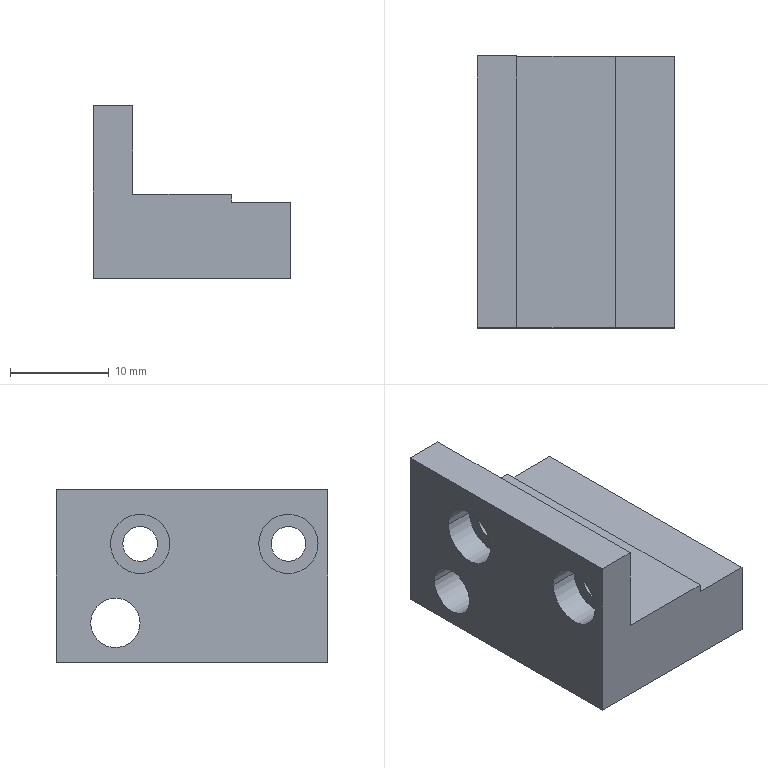Part | NX | 1 solid | 22 faces | box 20 x 27.5 x 17.5 mm | volume 4951 mm3 | plane 12 | cylinder 10 | commonest cylinder face diameters 3.5 x4 6 x4 5 x2
STEP:
#1=CARTESIAN_POINT('',(20.,5.5,-9.8));
#2=VERTEX_POINT('',#1);
#3=CARTESIAN_POINT('',(14.,5.5,-9.8));
#4=VERTEX_POINT('',#3);
#5=CARTESIAN_POINT('',(0.,5.5,-9.8));
#6=DIRECTION('',(-1.,0.,0.));
#7=VECTOR('',#6,1000.);
#8=LINE('',#5,#7);
#9=EDGE_CURVE('',#2,#4,#8,.T.);
#10=ORIENTED_EDGE('',*,*,#9,.T.);
#11=CARTESIAN_POINT('',(14.,5.5,-9.));
#12=VERTEX_POINT('',#11);
#13=CARTESIAN_POINT('',(14.,5.5,0.));
#14=DIRECTION('',(0.,0.,1.));
#15=VECTOR('',#14,1000.);
#16=LINE('',#13,#15);
#17=EDGE_CURVE('',#4,#12,#16,.T.);
#18=ORIENTED_EDGE('',*,*,#17,.T.);
#19=CARTESIAN_POINT('',(4.,5.5,-9.));
#20=VERTEX_POINT('',#19);
#21=CARTESIAN_POINT('',(0.,5.5,-9.));
#22=DIRECTION('',(1.,0.,0.));
#23=VECTOR('',#22,1000.);
#24=LINE('',#21,#23);
#25=EDGE_CURVE('',#20,#12,#24,.T.);
#26=ORIENTED_EDGE('',*,*,#25,.F.);
#27=CARTESIAN_POINT('',(4.,5.5,0.));
#28=VERTEX_POINT('',#27);
#29=CARTESIAN_POINT('',(4.,5.5,0.));
#30=DIRECTION('',(0.,0.,-1.));
#31=VECTOR('',#30,1000.);
#32=LINE('',#29,#31);
#33=EDGE_CURVE('',#28,#20,#32,.T.);
#34=ORIENTED_EDGE('',*,*,#33,.F.);
#35=CARTESIAN_POINT('',(0.,5.5,0.));
#36=VERTEX_POINT('',#35);
#37=CARTESIAN_POINT('',(0.,5.5,0.));
#38=DIRECTION('',(1.,0.,0.));
#39=VECTOR('',#38,1000.);
#40=LINE('',#37,#39);
#41=EDGE_CURVE('',#36,#28,#40,.T.);
#42=ORIENTED_EDGE('',*,*,#41,.F.);
#43=CARTESIAN_POINT('',(0.,5.5,-17.5));
#44=VERTEX_POINT('',#43);
#45=CARTESIAN_POINT('',(0.,5.5,0.));
#46=DIRECTION('',(0.,0.,1.));
#47=VECTOR('',#46,1000.);
#48=LINE('',#45,#47);
#49=EDGE_CURVE('',#44,#36,#48,.T.);
#50=ORIENTED_EDGE('',*,*,#49,.F.);
#51=CARTESIAN_POINT('',(20.,5.5,-17.5));
#52=VERTEX_POINT('',#51);
#53=CARTESIAN_POINT('',(0.,5.5,-17.5));
#54=DIRECTION('',(-1.,0.,0.));
#55=VECTOR('',#54,1000.);
#56=LINE('',#53,#55);
#57=EDGE_CURVE('',#52,#44,#56,.T.);
#58=ORIENTED_EDGE('',*,*,#57,.F.);
#59=CARTESIAN_POINT('',(20.,5.5,0.));
#60=DIRECTION('',(0.,0.,-1.));
#61=VECTOR('',#60,1000.);
#62=LINE('',#59,#61);
#63=EDGE_CURVE('',#2,#52,#62,.T.);
#64=ORIENTED_EDGE('',*,*,#63,.F.);
#65=EDGE_LOOP('',(#10,#18,#26,#34,#42,#50,#58,#64));
#66=FACE_BOUND('',#65,.T.);
#67=CARTESIAN_POINT('',(0.,5.5,0.));
#68=DIRECTION('',(0.,1.,0.));
#69=DIRECTION('',(1.,0.,0.));
#70=AXIS2_PLACEMENT_3D('',#67,#68,#69);
#71=PLANE('',#70);
#72=ADVANCED_FACE('',(#66),#71,.F.);
#73=ORIENTED_EDGE('',*,*,#9,.F.);
#74=CARTESIAN_POINT('',(20.,33.,-9.8));
#75=VERTEX_POINT('',#74);
#76=CARTESIAN_POINT('',(20.,0.,-9.8));
#77=DIRECTION('',(0.,-1.,0.));
#78=VECTOR('',#77,1000.);
#79=LINE('',#76,#78);
#80=EDGE_CURVE('',#75,#2,#79,.T.);
#81=ORIENTED_EDGE('',*,*,#80,.F.);
#82=CARTESIAN_POINT('',(14.,33.,-9.8));
#83=VERTEX_POINT('',#82);
#84=CARTESIAN_POINT('',(0.,33.,-9.8));
#85=DIRECTION('',(-1.,0.,0.));
#86=VECTOR('',#85,1000.);
#87=LINE('',#84,#86);
#88=EDGE_CURVE('',#75,#83,#87,.T.);
#89=ORIENTED_EDGE('',*,*,#88,.T.);
#90=CARTESIAN_POINT('',(14.,0.,-9.8));
#91=DIRECTION('',(0.,1.,0.));
#92=VECTOR('',#91,1000.);
#93=LINE('',#90,#92);
#94=EDGE_CURVE('',#4,#83,#93,.T.);
#95=ORIENTED_EDGE('',*,*,#94,.F.);
#96=EDGE_LOOP('',(#73,#81,#89,#95));
#97=FACE_BOUND('',#96,.T.);
#98=CARTESIAN_POINT('',(20.,34.,-9.8));
#99=DIRECTION('',(0.,0.,-1.));
#100=DIRECTION('',(0.,-1.,0.));
#101=AXIS2_PLACEMENT_3D('',#98,#99,#100);
#102=PLANE('',#101);
#103=ADVANCED_FACE('',(#97),#102,.F.);
#104=ORIENTED_EDGE('',*,*,#17,.F.);
#105=ORIENTED_EDGE('',*,*,#94,.T.);
#106=CARTESIAN_POINT('',(14.,33.,-9.));
#107=VERTEX_POINT('',#106);
#108=CARTESIAN_POINT('',(14.,33.,0.));
#109=DIRECTION('',(0.,0.,1.));
#110=VECTOR('',#109,1000.);
#111=LINE('',#108,#110);
#112=EDGE_CURVE('',#83,#107,#111,.T.);
#113=ORIENTED_EDGE('',*,*,#112,.T.);
#114=CARTESIAN_POINT('',(14.,0.,-9.));
#115=DIRECTION('',(0.,-1.,0.));
#116=VECTOR('',#115,1000.);
#117=LINE('',#114,#116);
#118=EDGE_CURVE('',#107,#12,#117,.T.);
#119=ORIENTED_EDGE('',*,*,#118,.T.);
#120=EDGE_LOOP('',(#104,#105,#113,#119));
#121=FACE_BOUND('',#120,.T.);
#122=CARTESIAN_POINT('',(14.,34.,-9.8));
#123=DIRECTION('',(-1.,0.,0.));
#124=DIRECTION('',(0.,0.,1.));
#125=AXIS2_PLACEMENT_3D('',#122,#123,#124);
#126=PLANE('',#125);
#127=ADVANCED_FACE('',(#121),#126,.F.);
#128=ORIENTED_EDGE('',*,*,#118,.F.);
#129=CARTESIAN_POINT('',(4.,33.,-9.));
#130=VERTEX_POINT('',#129);
#131=CARTESIAN_POINT('',(0.,33.,-9.));
#132=DIRECTION('',(1.,0.,0.));
#133=VECTOR('',#132,1000.);
#134=LINE('',#131,#133);
#135=EDGE_CURVE('',#130,#107,#134,.T.);
#136=ORIENTED_EDGE('',*,*,#135,.F.);
#137=CARTESIAN_POINT('',(4.,0.,-9.));
#138=DIRECTION('',(0.,1.,0.));
#139=VECTOR('',#138,1000.);
#140=LINE('',#137,#139);
#141=EDGE_CURVE('',#20,#130,#140,.T.);
#142=ORIENTED_EDGE('',*,*,#141,.F.);
#143=ORIENTED_EDGE('',*,*,#25,.T.);
#144=EDGE_LOOP('',(#128,#136,#142,#143));
#145=FACE_BOUND('',#144,.T.);
#146=CARTESIAN_POINT('',(4.,0.,-9.));
#147=DIRECTION('',(0.,0.,1.));
#148=DIRECTION('',(1.,0.,0.));
#149=AXIS2_PLACEMENT_3D('',#146,#147,#148);
#150=PLANE('',#149);
#151=ADVANCED_FACE('',(#145),#150,.T.);
#152=ORIENTED_EDGE('',*,*,#80,.T.);
#153=ORIENTED_EDGE('',*,*,#63,.T.);
#154=CARTESIAN_POINT('',(20.,33.,-17.5));
#155=VERTEX_POINT('',#154);
#156=CARTESIAN_POINT('',(20.,0.,-17.5));
#157=DIRECTION('',(0.,-1.,0.));
#158=VECTOR('',#157,1000.);
#159=LINE('',#156,#158);
#160=EDGE_CURVE('',#155,#52,#159,.T.);
#161=ORIENTED_EDGE('',*,*,#160,.F.);
#162=CARTESIAN_POINT('',(20.,33.,0.));
#163=DIRECTION('',(0.,0.,-1.));
#164=VECTOR('',#163,1000.);
#165=LINE('',#162,#164);
#166=EDGE_CURVE('',#75,#155,#165,.T.);
#167=ORIENTED_EDGE('',*,*,#166,.F.);
#168=EDGE_LOOP('',(#152,#153,#161,#167));
#169=FACE_BOUND('',#168,.T.);
#170=CARTESIAN_POINT('',(20.,29.5,-13.5));
#171=VERTEX_POINT('',#170);
#172=CARTESIAN_POINT('',(20.,24.5,-13.5));
#173=VERTEX_POINT('',#172);
#174=CARTESIAN_POINT('',(20.,27.,-13.5));
#175=DIRECTION('',(1.,0.,0.));
#176=DIRECTION('',(0.,1.,0.));
#177=AXIS2_PLACEMENT_3D('',#174,#175,#176);
#178=CIRCLE('',#177,2.5);
#179=EDGE_CURVE('',#171,#173,#178,.T.);
#180=ORIENTED_EDGE('',*,*,#179,.F.);
#181=CARTESIAN_POINT('',(20.,27.,-13.5));
#182=DIRECTION('',(1.,0.,0.));
#183=DIRECTION('',(0.,1.,0.));
#184=AXIS2_PLACEMENT_3D('',#181,#182,#183);
#185=CIRCLE('',#184,2.5);
#186=EDGE_CURVE('',#173,#171,#185,.T.);
#187=ORIENTED_EDGE('',*,*,#186,.F.);
#188=EDGE_LOOP('',(#180,#187));
#189=FACE_BOUND('',#188,.T.);
#190=CARTESIAN_POINT('',(20.,0.,-9.));
#191=DIRECTION('',(1.,0.,0.));
#192=DIRECTION('',(0.,1.,0.));
#193=AXIS2_PLACEMENT_3D('',#190,#191,#192);
#194=PLANE('',#193);
#195=ADVANCED_FACE('',(#169,#189),#194,.T.);
#196=ORIENTED_EDGE('',*,*,#41,.T.);
#197=CARTESIAN_POINT('',(4.,33.,0.));
#198=VERTEX_POINT('',#197);
#199=CARTESIAN_POINT('',(4.,0.,0.));
#200=DIRECTION('',(0.,-1.,0.));
#201=VECTOR('',#200,1000.);
#202=LINE('',#199,#201);
#203=EDGE_CURVE('',#198,#28,#202,.T.);
#204=ORIENTED_EDGE('',*,*,#203,.F.);
#205=CARTESIAN_POINT('',(0.,33.,0.));
#206=VERTEX_POINT('',#205);
#207=CARTESIAN_POINT('',(0.,33.,0.));
#208=DIRECTION('',(1.,0.,0.));
#209=VECTOR('',#208,1000.);
#210=LINE('',#207,#209);
#211=EDGE_CURVE('',#206,#198,#210,.T.);
#212=ORIENTED_EDGE('',*,*,#211,.F.);
#213=CARTESIAN_POINT('',(0.,0.,0.));
#214=DIRECTION('',(0.,1.,0.));
#215=VECTOR('',#214,1000.);
#216=LINE('',#213,#215);
#217=EDGE_CURVE('',#36,#206,#216,.T.);
#218=ORIENTED_EDGE('',*,*,#217,.F.);
#219=EDGE_LOOP('',(#196,#204,#212,#218));
#220=FACE_BOUND('',#219,.T.);
#221=CARTESIAN_POINT('',(0.,0.,0.));
#222=DIRECTION('',(0.,0.,1.));
#223=DIRECTION('',(1.,0.,0.));
#224=AXIS2_PLACEMENT_3D('',#221,#222,#223);
#225=PLANE('',#224);
#226=ADVANCED_FACE('',(#220),#225,.T.);
#227=ORIENTED_EDGE('',*,*,#33,.T.);
#228=ORIENTED_EDGE('',*,*,#141,.T.);
#229=CARTESIAN_POINT('',(4.,33.,0.));
#230=DIRECTION('',(0.,0.,-1.));
#231=VECTOR('',#230,1000.);
#232=LINE('',#229,#231);
#233=EDGE_CURVE('',#198,#130,#232,.T.);
#234=ORIENTED_EDGE('',*,*,#233,.F.);
#235=ORIENTED_EDGE('',*,*,#203,.T.);
#236=EDGE_LOOP('',(#227,#228,#234,#235));
#237=FACE_BOUND('',#236,.T.);
#238=CARTESIAN_POINT('',(4.,7.75,-5.5));
#239=VERTEX_POINT('',#238);
#240=CARTESIAN_POINT('',(4.,11.25,-5.5));
#241=VERTEX_POINT('',#240);
#242=CARTESIAN_POINT('',(4.,9.5,-5.5));
#243=DIRECTION('',(-1.,0.,0.));
#244=DIRECTION('',(0.,1.,0.));
#245=AXIS2_PLACEMENT_3D('',#242,#243,#244);
#246=CIRCLE('',#245,1.75);
#247=EDGE_CURVE('',#239,#241,#246,.T.);
#248=ORIENTED_EDGE('',*,*,#247,.T.);
#249=CARTESIAN_POINT('',(4.,9.5,-5.5));
#250=DIRECTION('',(-1.,0.,0.));
#251=DIRECTION('',(0.,1.,0.));
#252=AXIS2_PLACEMENT_3D('',#249,#250,#251);
#253=CIRCLE('',#252,1.75);
#254=EDGE_CURVE('',#241,#239,#253,.T.);
#255=ORIENTED_EDGE('',*,*,#254,.T.);
#256=EDGE_LOOP('',(#248,#255));
#257=FACE_BOUND('',#256,.T.);
#258=CARTESIAN_POINT('',(4.,26.25,-5.5));
#259=VERTEX_POINT('',#258);
#260=CARTESIAN_POINT('',(4.,22.75,-5.5));
#261=VERTEX_POINT('',#260);
#262=CARTESIAN_POINT('',(4.,24.5,-5.5));
#263=DIRECTION('',(-1.,0.,0.));
#264=DIRECTION('',(0.,1.,0.));
#265=AXIS2_PLACEMENT_3D('',#262,#263,#264);
#266=CIRCLE('',#265,1.75);
#267=EDGE_CURVE('',#259,#261,#266,.T.);
#268=ORIENTED_EDGE('',*,*,#267,.T.);
#269=CARTESIAN_POINT('',(4.,24.5,-5.5));
#270=DIRECTION('',(-1.,0.,0.));
#271=DIRECTION('',(0.,1.,0.));
#272=AXIS2_PLACEMENT_3D('',#269,#270,#271);
#273=CIRCLE('',#272,1.75);
#274=EDGE_CURVE('',#261,#259,#273,.T.);
#275=ORIENTED_EDGE('',*,*,#274,.T.);
#276=EDGE_LOOP('',(#268,#275));
#277=FACE_BOUND('',#276,.T.);
#278=CARTESIAN_POINT('',(4.,0.,0.));
#279=DIRECTION('',(1.,0.,0.));
#280=DIRECTION('',(0.,1.,0.));
#281=AXIS2_PLACEMENT_3D('',#278,#279,#280);
#282=PLANE('',#281);
#283=ADVANCED_FACE('',(#237,#257,#277),#282,.T.);
#284=ORIENTED_EDGE('',*,*,#57,.T.);
#285=CARTESIAN_POINT('',(0.,33.,-17.5));
#286=VERTEX_POINT('',#285);
#287=CARTESIAN_POINT('',(0.,0.,-17.5));
#288=DIRECTION('',(0.,-1.,0.));
#289=VECTOR('',#288,1000.);
#290=LINE('',#287,#289);
#291=EDGE_CURVE('',#286,#44,#290,.T.);
#292=ORIENTED_EDGE('',*,*,#291,.F.);
#293=CARTESIAN_POINT('',(0.,33.,-17.5));
#294=DIRECTION('',(-1.,0.,0.));
#295=VECTOR('',#294,1000.);
#296=LINE('',#293,#295);
#297=EDGE_CURVE('',#155,#286,#296,.T.);
#298=ORIENTED_EDGE('',*,*,#297,.F.);
#299=ORIENTED_EDGE('',*,*,#160,.T.);
#300=EDGE_LOOP('',(#284,#292,#298,#299));
#301=FACE_BOUND('',#300,.T.);
#302=CARTESIAN_POINT('',(20.,0.,-17.5));
#303=DIRECTION('',(0.,0.,-1.));
#304=DIRECTION('',(0.,-1.,0.));
#305=AXIS2_PLACEMENT_3D('',#302,#303,#304);
#306=PLANE('',#305);
#307=ADVANCED_FACE('',(#301),#306,.T.);
#308=ORIENTED_EDGE('',*,*,#49,.T.);
#309=ORIENTED_EDGE('',*,*,#217,.T.);
#310=CARTESIAN_POINT('',(0.,33.,0.));
#311=DIRECTION('',(0.,0.,1.));
#312=VECTOR('',#311,1000.);
#313=LINE('',#310,#312);
#314=EDGE_CURVE('',#286,#206,#313,.T.);
#315=ORIENTED_EDGE('',*,*,#314,.F.);
#316=ORIENTED_EDGE('',*,*,#291,.T.);
#317=EDGE_LOOP('',(#308,#309,#315,#316));
#318=FACE_BOUND('',#317,.T.);
#319=CARTESIAN_POINT('',(0.,12.5,-5.5));
#320=VERTEX_POINT('',#319);
#321=CARTESIAN_POINT('',(0.,6.5,-5.5));
#322=VERTEX_POINT('',#321);
#323=CARTESIAN_POINT('',(0.,9.5,-5.5));
#324=DIRECTION('',(-1.,0.,0.));
#325=DIRECTION('',(0.,1.,0.));
#326=AXIS2_PLACEMENT_3D('',#323,#324,#325);
#327=CIRCLE('',#326,3.);
#328=EDGE_CURVE('',#320,#322,#327,.T.);
#329=ORIENTED_EDGE('',*,*,#328,.F.);
#330=CARTESIAN_POINT('',(0.,9.5,-5.5));
#331=DIRECTION('',(-1.,0.,0.));
#332=DIRECTION('',(0.,1.,0.));
#333=AXIS2_PLACEMENT_3D('',#330,#331,#332);
#334=CIRCLE('',#333,3.);
#335=EDGE_CURVE('',#322,#320,#334,.T.);
#336=ORIENTED_EDGE('',*,*,#335,.F.);
#337=EDGE_LOOP('',(#329,#336));
#338=FACE_BOUND('',#337,.T.);
#339=CARTESIAN_POINT('',(0.,24.5,-13.5));
#340=VERTEX_POINT('',#339);
#341=CARTESIAN_POINT('',(0.,29.5,-13.5));
#342=VERTEX_POINT('',#341);
#343=CARTESIAN_POINT('',(0.,27.,-13.5));
#344=DIRECTION('',(1.,0.,0.));
#345=DIRECTION('',(0.,1.,0.));
#346=AXIS2_PLACEMENT_3D('',#343,#344,#345);
#347=CIRCLE('',#346,2.5);
#348=EDGE_CURVE('',#340,#342,#347,.T.);
#349=ORIENTED_EDGE('',*,*,#348,.T.);
#350=CARTESIAN_POINT('',(0.,27.,-13.5));
#351=DIRECTION('',(1.,0.,0.));
#352=DIRECTION('',(0.,1.,0.));
#353=AXIS2_PLACEMENT_3D('',#350,#351,#352);
#354=CIRCLE('',#353,2.5);
#355=EDGE_CURVE('',#342,#340,#354,.T.);
#356=ORIENTED_EDGE('',*,*,#355,.T.);
#357=EDGE_LOOP('',(#349,#356));
#358=FACE_BOUND('',#357,.T.);
#359=CARTESIAN_POINT('',(0.,21.5,-5.5));
#360=VERTEX_POINT('',#359);
#361=CARTESIAN_POINT('',(0.,27.5,-5.5));
#362=VERTEX_POINT('',#361);
#363=CARTESIAN_POINT('',(0.,24.5,-5.5));
#364=DIRECTION('',(-1.,0.,0.));
#365=DIRECTION('',(0.,1.,0.));
#366=AXIS2_PLACEMENT_3D('',#363,#364,#365);
#367=CIRCLE('',#366,3.);
#368=EDGE_CURVE('',#360,#362,#367,.T.);
#369=ORIENTED_EDGE('',*,*,#368,.F.);
#370=CARTESIAN_POINT('',(0.,24.5,-5.5));
#371=DIRECTION('',(-1.,0.,0.));
#372=DIRECTION('',(0.,1.,0.));
#373=AXIS2_PLACEMENT_3D('',#370,#371,#372);
#374=CIRCLE('',#373,3.);
#375=EDGE_CURVE('',#362,#360,#374,.T.);
#376=ORIENTED_EDGE('',*,*,#375,.F.);
#377=EDGE_LOOP('',(#369,#376));
#378=FACE_BOUND('',#377,.T.);
#379=CARTESIAN_POINT('',(0.,0.,-17.5));
#380=DIRECTION('',(-1.,0.,0.));
#381=DIRECTION('',(0.,0.,1.));
#382=AXIS2_PLACEMENT_3D('',#379,#380,#381);
#383=PLANE('',#382);
#384=ADVANCED_FACE('',(#318,#338,#358,#378),#383,.T.);
#385=ORIENTED_EDGE('',*,*,#88,.F.);
#386=ORIENTED_EDGE('',*,*,#166,.T.);
#387=ORIENTED_EDGE('',*,*,#297,.T.);
#388=ORIENTED_EDGE('',*,*,#314,.T.);
#389=ORIENTED_EDGE('',*,*,#211,.T.);
#390=ORIENTED_EDGE('',*,*,#233,.T.);
#391=ORIENTED_EDGE('',*,*,#135,.T.);
#392=ORIENTED_EDGE('',*,*,#112,.F.);
#393=EDGE_LOOP('',(#385,#386,#387,#388,#389,#390,#391,#392));
#394=FACE_BOUND('',#393,.T.);
#395=CARTESIAN_POINT('',(0.,33.,0.));
#396=DIRECTION('',(0.,1.,0.));
#397=DIRECTION('',(1.,0.,0.));
#398=AXIS2_PLACEMENT_3D('',#395,#396,#397);
#399=PLANE('',#398);
#400=ADVANCED_FACE('',(#394),#399,.T.);
#401=ORIENTED_EDGE('',*,*,#179,.T.);
#402=CARTESIAN_POINT('',(0.,24.5,-13.5));
#403=DIRECTION('',(1.,0.,0.));
#404=VECTOR('',#403,1000.);
#405=LINE('',#402,#404);
#406=EDGE_CURVE('',#173,#340,#405,.F.);
#407=ORIENTED_EDGE('',*,*,#406,.T.);
#408=ORIENTED_EDGE('',*,*,#355,.F.);
#409=CARTESIAN_POINT('',(0.,29.5,-13.5));
#410=DIRECTION('',(1.,0.,0.));
#411=VECTOR('',#410,1000.);
#412=LINE('',#409,#411);
#413=EDGE_CURVE('',#171,#342,#412,.F.);
#414=ORIENTED_EDGE('',*,*,#413,.F.);
#415=EDGE_LOOP('',(#401,#407,#408,#414));
#416=FACE_BOUND('',#415,.T.);
#417=CARTESIAN_POINT('',(0.,27.,-13.5));
#418=DIRECTION('',(1.,0.,0.));
#419=DIRECTION('',(0.,1.,0.));
#420=AXIS2_PLACEMENT_3D('',#417,#418,#419);
#421=CYLINDRICAL_SURFACE('',#420,2.5);
#422=ADVANCED_FACE('',(#416),#421,.F.);
#423=ORIENTED_EDGE('',*,*,#368,.T.);
#424=CARTESIAN_POINT('',(3.,27.5,-5.5));
#425=VERTEX_POINT('',#424);
#426=CARTESIAN_POINT('',(23.1,27.5,-5.5));
#427=DIRECTION('',(-1.,0.,0.));
#428=VECTOR('',#427,1000.);
#429=LINE('',#426,#428);
#430=EDGE_CURVE('',#425,#362,#429,.T.);
#431=ORIENTED_EDGE('',*,*,#430,.F.);
#432=CARTESIAN_POINT('',(3.,21.5,-5.5));
#433=VERTEX_POINT('',#432);
#434=CARTESIAN_POINT('',(3.,24.5,-5.5));
#435=DIRECTION('',(1.,0.,0.));
#436=DIRECTION('',(0.,1.,0.));
#437=AXIS2_PLACEMENT_3D('',#434,#435,#436);
#438=CIRCLE('',#437,3.);
#439=EDGE_CURVE('',#425,#433,#438,.T.);
#440=ORIENTED_EDGE('',*,*,#439,.T.);
#441=CARTESIAN_POINT('',(23.1,21.5,-5.5));
#442=DIRECTION('',(-1.,0.,0.));
#443=VECTOR('',#442,1000.);
#444=LINE('',#441,#443);
#445=EDGE_CURVE('',#433,#360,#444,.T.);
#446=ORIENTED_EDGE('',*,*,#445,.T.);
#447=EDGE_LOOP('',(#423,#431,#440,#446));
#448=FACE_BOUND('',#447,.T.);
#449=CARTESIAN_POINT('',(23.1,24.5,-5.5));
#450=DIRECTION('',(-1.,0.,0.));
#451=DIRECTION('',(0.,1.,0.));
#452=AXIS2_PLACEMENT_3D('',#449,#450,#451);
#453=CYLINDRICAL_SURFACE('',#452,3.);
#454=ADVANCED_FACE('',(#448),#453,.F.);
#455=CARTESIAN_POINT('',(3.,12.5,-5.5));
#456=VERTEX_POINT('',#455);
#457=CARTESIAN_POINT('',(3.,6.5,-5.5));
#458=VERTEX_POINT('',#457);
#459=CARTESIAN_POINT('',(3.,9.5,-5.5));
#460=DIRECTION('',(1.,0.,0.));
#461=DIRECTION('',(0.,1.,0.));
#462=AXIS2_PLACEMENT_3D('',#459,#460,#461);
#463=CIRCLE('',#462,3.);
#464=EDGE_CURVE('',#456,#458,#463,.T.);
#465=ORIENTED_EDGE('',*,*,#464,.T.);
#466=CARTESIAN_POINT('',(23.1,6.5,-5.5));
#467=DIRECTION('',(-1.,0.,0.));
#468=VECTOR('',#467,1000.);
#469=LINE('',#466,#468);
#470=EDGE_CURVE('',#322,#458,#469,.F.);
#471=ORIENTED_EDGE('',*,*,#470,.F.);
#472=ORIENTED_EDGE('',*,*,#335,.T.);
#473=CARTESIAN_POINT('',(23.1,12.5,-5.5));
#474=DIRECTION('',(-1.,0.,0.));
#475=VECTOR('',#474,1000.);
#476=LINE('',#473,#475);
#477=EDGE_CURVE('',#320,#456,#476,.F.);
#478=ORIENTED_EDGE('',*,*,#477,.T.);
#479=EDGE_LOOP('',(#465,#471,#472,#478));
#480=FACE_BOUND('',#479,.T.);
#481=CARTESIAN_POINT('',(23.1,9.5,-5.5));
#482=DIRECTION('',(-1.,0.,0.));
#483=DIRECTION('',(0.,1.,0.));
#484=AXIS2_PLACEMENT_3D('',#481,#482,#483);
#485=CYLINDRICAL_SURFACE('',#484,3.);
#486=ADVANCED_FACE('',(#480),#485,.F.);
#487=ORIENTED_EDGE('',*,*,#439,.F.);
#488=CARTESIAN_POINT('',(3.,24.5,-5.5));
#489=DIRECTION('',(1.,0.,0.));
#490=DIRECTION('',(0.,1.,0.));
#491=AXIS2_PLACEMENT_3D('',#488,#489,#490);
#492=CIRCLE('',#491,3.);
#493=EDGE_CURVE('',#433,#425,#492,.T.);
#494=ORIENTED_EDGE('',*,*,#493,.F.);
#495=EDGE_LOOP('',(#487,#494));
#496=FACE_BOUND('',#495,.T.);
#497=CARTESIAN_POINT('',(3.,26.25,-5.5));
#498=VERTEX_POINT('',#497);
#499=CARTESIAN_POINT('',(3.,22.75,-5.5));
#500=VERTEX_POINT('',#499);
#501=CARTESIAN_POINT('',(3.,24.5,-5.5));
#502=DIRECTION('',(-1.,0.,0.));
#503=DIRECTION('',(0.,1.,0.));
#504=AXIS2_PLACEMENT_3D('',#501,#502,#503);
#505=CIRCLE('',#504,1.75);
#506=EDGE_CURVE('',#498,#500,#505,.T.);
#507=ORIENTED_EDGE('',*,*,#506,.F.);
#508=CARTESIAN_POINT('',(3.,24.5,-5.5));
#509=DIRECTION('',(-1.,0.,0.));
#510=DIRECTION('',(0.,1.,0.));
#511=AXIS2_PLACEMENT_3D('',#508,#509,#510);
#512=CIRCLE('',#511,1.75);
#513=EDGE_CURVE('',#500,#498,#512,.T.);
#514=ORIENTED_EDGE('',*,*,#513,.F.);
#515=EDGE_LOOP('',(#507,#514));
#516=FACE_BOUND('',#515,.T.);
#517=CARTESIAN_POINT('',(3.,24.5,-5.5));
#518=DIRECTION('',(-1.,0.,0.));
#519=DIRECTION('',(0.,0.,1.));
#520=AXIS2_PLACEMENT_3D('',#517,#518,#519);
#521=PLANE('',#520);
#522=ADVANCED_FACE('',(#496,#516),#521,.T.);
#523=ORIENTED_EDGE('',*,*,#464,.F.);
#524=CARTESIAN_POINT('',(3.,9.5,-5.5));
#525=DIRECTION('',(1.,0.,0.));
#526=DIRECTION('',(0.,1.,0.));
#527=AXIS2_PLACEMENT_3D('',#524,#525,#526);
#528=CIRCLE('',#527,3.);
#529=EDGE_CURVE('',#458,#456,#528,.T.);
#530=ORIENTED_EDGE('',*,*,#529,.F.);
#531=EDGE_LOOP('',(#523,#530));
#532=FACE_BOUND('',#531,.T.);
#533=CARTESIAN_POINT('',(3.,11.25,-5.5));
#534=VERTEX_POINT('',#533);
#535=CARTESIAN_POINT('',(3.,7.75,-5.5));
#536=VERTEX_POINT('',#535);
#537=CARTESIAN_POINT('',(3.,9.5,-5.5));
#538=DIRECTION('',(-1.,0.,0.));
#539=DIRECTION('',(0.,1.,0.));
#540=AXIS2_PLACEMENT_3D('',#537,#538,#539);
#541=CIRCLE('',#540,1.75);
#542=EDGE_CURVE('',#534,#536,#541,.T.);
#543=ORIENTED_EDGE('',*,*,#542,.F.);
#544=CARTESIAN_POINT('',(3.,9.5,-5.5));
#545=DIRECTION('',(-1.,0.,0.));
#546=DIRECTION('',(0.,1.,0.));
#547=AXIS2_PLACEMENT_3D('',#544,#545,#546);
#548=CIRCLE('',#547,1.75);
#549=EDGE_CURVE('',#536,#534,#548,.T.);
#550=ORIENTED_EDGE('',*,*,#549,.F.);
#551=EDGE_LOOP('',(#543,#550));
#552=FACE_BOUND('',#551,.T.);
#553=CARTESIAN_POINT('',(3.,9.5,-5.5));
#554=DIRECTION('',(-1.,0.,0.));
#555=DIRECTION('',(0.,0.,1.));
#556=AXIS2_PLACEMENT_3D('',#553,#554,#555);
#557=PLANE('',#556);
#558=ADVANCED_FACE('',(#532,#552),#557,.T.);
#559=ORIENTED_EDGE('',*,*,#542,.T.);
#560=CARTESIAN_POINT('',(23.1,7.75,-5.5));
#561=DIRECTION('',(-1.,0.,0.));
#562=VECTOR('',#561,1000.);
#563=LINE('',#560,#562);
#564=EDGE_CURVE('',#536,#239,#563,.F.);
#565=ORIENTED_EDGE('',*,*,#564,.T.);
#566=ORIENTED_EDGE('',*,*,#254,.F.);
#567=CARTESIAN_POINT('',(23.1,11.25,-5.5));
#568=DIRECTION('',(-1.,0.,0.));
#569=VECTOR('',#568,1000.);
#570=LINE('',#567,#569);
#571=EDGE_CURVE('',#534,#241,#570,.F.);
#572=ORIENTED_EDGE('',*,*,#571,.F.);
#573=EDGE_LOOP('',(#559,#565,#566,#572));
#574=FACE_BOUND('',#573,.T.);
#575=CARTESIAN_POINT('',(23.1,9.5,-5.5));
#576=DIRECTION('',(-1.,0.,0.));
#577=DIRECTION('',(0.,1.,0.));
#578=AXIS2_PLACEMENT_3D('',#575,#576,#577);
#579=CYLINDRICAL_SURFACE('',#578,1.75);
#580=ADVANCED_FACE('',(#574),#579,.F.);
#581=ORIENTED_EDGE('',*,*,#267,.F.);
#582=CARTESIAN_POINT('',(23.1,26.25,-5.5));
#583=DIRECTION('',(-1.,0.,0.));
#584=VECTOR('',#583,1000.);
#585=LINE('',#582,#584);
#586=EDGE_CURVE('',#259,#498,#585,.T.);
#587=ORIENTED_EDGE('',*,*,#586,.T.);
#588=ORIENTED_EDGE('',*,*,#506,.T.);
#589=CARTESIAN_POINT('',(23.1,22.75,-5.5));
#590=DIRECTION('',(-1.,0.,0.));
#591=VECTOR('',#590,1000.);
#592=LINE('',#589,#591);
#593=EDGE_CURVE('',#261,#500,#592,.T.);
#594=ORIENTED_EDGE('',*,*,#593,.F.);
#595=EDGE_LOOP('',(#581,#587,#588,#594));
#596=FACE_BOUND('',#595,.T.);
#597=CARTESIAN_POINT('',(23.1,24.5,-5.5));
#598=DIRECTION('',(-1.,0.,0.));
#599=DIRECTION('',(0.,1.,0.));
#600=AXIS2_PLACEMENT_3D('',#597,#598,#599);
#601=CYLINDRICAL_SURFACE('',#600,1.75);
#602=ADVANCED_FACE('',(#596),#601,.F.);
#603=ORIENTED_EDGE('',*,*,#247,.F.);
#604=ORIENTED_EDGE('',*,*,#564,.F.);
#605=ORIENTED_EDGE('',*,*,#549,.T.);
#606=ORIENTED_EDGE('',*,*,#571,.T.);
#607=EDGE_LOOP('',(#603,#604,#605,#606));
#608=FACE_BOUND('',#607,.T.);
#609=CARTESIAN_POINT('',(23.1,9.5,-5.5));
#610=DIRECTION('',(-1.,0.,0.));
#611=DIRECTION('',(0.,1.,0.));
#612=AXIS2_PLACEMENT_3D('',#609,#610,#611);
#613=CYLINDRICAL_SURFACE('',#612,1.75);
#614=ADVANCED_FACE('',(#608),#613,.F.);
#615=ORIENTED_EDGE('',*,*,#430,.T.);
#616=ORIENTED_EDGE('',*,*,#375,.T.);
#617=ORIENTED_EDGE('',*,*,#445,.F.);
#618=ORIENTED_EDGE('',*,*,#493,.T.);
#619=EDGE_LOOP('',(#615,#616,#617,#618));
#620=FACE_BOUND('',#619,.T.);
#621=CARTESIAN_POINT('',(23.1,24.5,-5.5));
#622=DIRECTION('',(-1.,0.,0.));
#623=DIRECTION('',(0.,1.,0.));
#624=AXIS2_PLACEMENT_3D('',#621,#622,#623);
#625=CYLINDRICAL_SURFACE('',#624,3.);
#626=ADVANCED_FACE('',(#620),#625,.F.);
#627=ORIENTED_EDGE('',*,*,#586,.F.);
#628=ORIENTED_EDGE('',*,*,#274,.F.);
#629=ORIENTED_EDGE('',*,*,#593,.T.);
#630=ORIENTED_EDGE('',*,*,#513,.T.);
#631=EDGE_LOOP('',(#627,#628,#629,#630));
#632=FACE_BOUND('',#631,.T.);
#633=CARTESIAN_POINT('',(23.1,24.5,-5.5));
#634=DIRECTION('',(-1.,0.,0.));
#635=DIRECTION('',(0.,1.,0.));
#636=AXIS2_PLACEMENT_3D('',#633,#634,#635);
#637=CYLINDRICAL_SURFACE('',#636,1.75);
#638=ADVANCED_FACE('',(#632),#637,.F.);
#639=ORIENTED_EDGE('',*,*,#328,.T.);
#640=ORIENTED_EDGE('',*,*,#470,.T.);
#641=ORIENTED_EDGE('',*,*,#529,.T.);
#642=ORIENTED_EDGE('',*,*,#477,.F.);
#643=EDGE_LOOP('',(#639,#640,#641,#642));
#644=FACE_BOUND('',#643,.T.);
#645=CARTESIAN_POINT('',(23.1,9.5,-5.5));
#646=DIRECTION('',(-1.,0.,0.));
#647=DIRECTION('',(0.,1.,0.));
#648=AXIS2_PLACEMENT_3D('',#645,#646,#647);
#649=CYLINDRICAL_SURFACE('',#648,3.);
#650=ADVANCED_FACE('',(#644),#649,.F.);
#651=ORIENTED_EDGE('',*,*,#348,.F.);
#652=ORIENTED_EDGE('',*,*,#406,.F.);
#653=ORIENTED_EDGE('',*,*,#186,.T.);
#654=ORIENTED_EDGE('',*,*,#413,.T.);
#655=EDGE_LOOP('',(#651,#652,#653,#654));
#656=FACE_BOUND('',#655,.T.);
#657=CARTESIAN_POINT('',(0.,27.,-13.5));
#658=DIRECTION('',(1.,0.,0.));
#659=DIRECTION('',(0.,1.,0.));
#660=AXIS2_PLACEMENT_3D('',#657,#658,#659);
#661=CYLINDRICAL_SURFACE('',#660,2.5);
#662=ADVANCED_FACE('',(#656),#661,.F.);
#663=CLOSED_SHELL('',(#72,#103,#127,#151,#195,#226,#283,#307,#384,#400,#422,#454,#486,#522,#558,#580,#602,#614,#626,#638,#650,#662));
#664=MANIFOLD_SOLID_BREP('',#663);
#665=(LENGTH_UNIT()NAMED_UNIT(*)SI_UNIT(.MILLI.,.METRE.));
#666=UNCERTAINTY_MEASURE_WITH_UNIT(LENGTH_MEASURE(0.00001),#665,'','');
#667=(NAMED_UNIT(*)PLANE_ANGLE_UNIT()SI_UNIT($,.RADIAN.));
#668=(NAMED_UNIT(*)SI_UNIT($,.STERADIAN.)SOLID_ANGLE_UNIT());
#669=(GEOMETRIC_REPRESENTATION_CONTEXT(3)GLOBAL_UNCERTAINTY_ASSIGNED_CONTEXT((#666))GLOBAL_UNIT_ASSIGNED_CONTEXT((#665,#667,#668))REPRESENTATION_CONTEXT('',''));
#670=ADVANCED_BREP_SHAPE_REPRESENTATION('',(#664),#669);